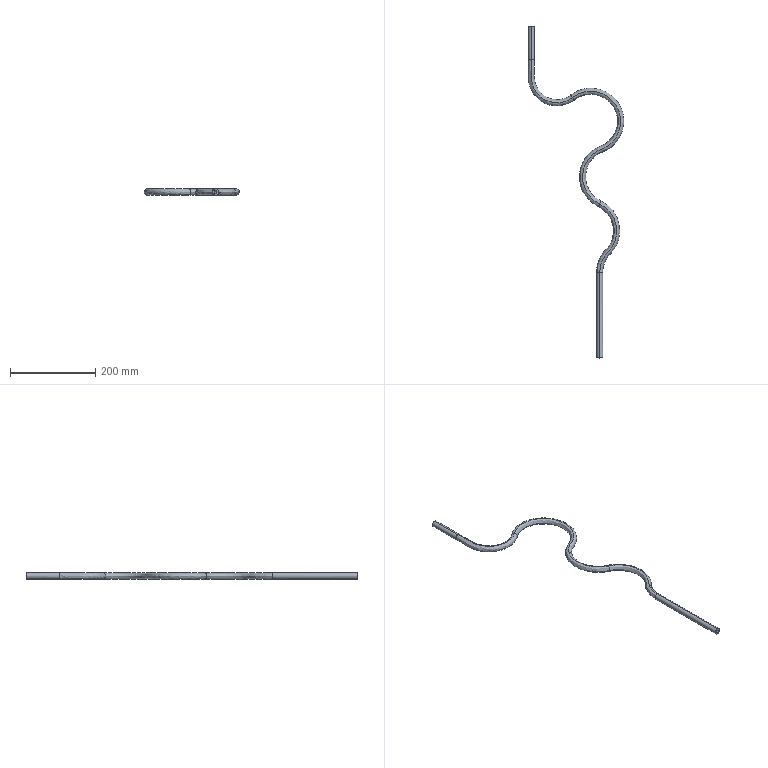Part | NX | features BREP 1 | 1 solid | 23 faces | box 223.745 x 778 x 14.512 mm | volume 139309 mm3 | spline 12 | cylinder 9 | plane 2 | commonest cylinder face diameters 6.35 x5 14.5 x4